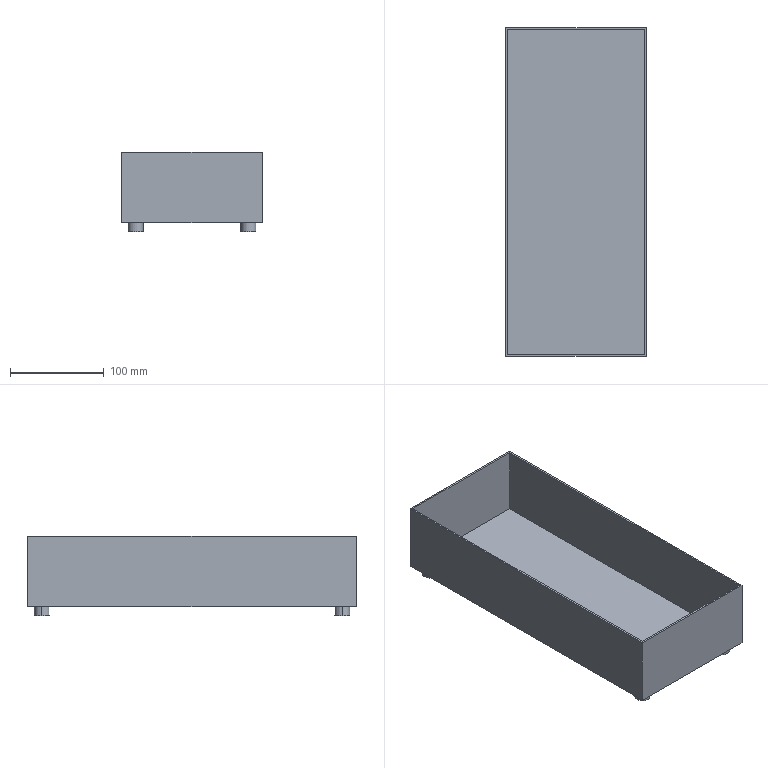Part | SolidWorks | features Extrusion 1, ICE 1, Shell 1 | 1 solid | 51 faces | box 150 x 350 x 85 mm | volume 254199 mm3 | plane 43 | cylinder 8 | commonest cylinder face diameters 16 x8
STEP:
#1=CARTESIAN_POINT('',(-68.,160.,-10.));
#2=VERTEX_POINT('',#1);
#3=CARTESIAN_POINT('',(-52.,160.,-10.));
#4=VERTEX_POINT('',#3);
#5=CARTESIAN_POINT('',(-60.,160.,-10.));
#6=DIRECTION('',(0.,0.,-1.));
#7=DIRECTION('',(1.,0.,0.));
#8=AXIS2_PLACEMENT_3D('',#5,#6,#7);
#9=CIRCLE('',#8,8.);
#10=EDGE_CURVE('',#2,#4,#9,.T.);
#11=ORIENTED_EDGE('',*,*,#10,.F.);
#12=CARTESIAN_POINT('',(-68.,160.,0.));
#13=VERTEX_POINT('',#12);
#14=CARTESIAN_POINT('',(-68.,160.,-10.));
#15=DIRECTION('',(0.,0.,1.));
#16=VECTOR('',#15,1000.);
#17=LINE('',#14,#16);
#18=EDGE_CURVE('',#2,#13,#17,.T.);
#19=ORIENTED_EDGE('',*,*,#18,.T.);
#20=CARTESIAN_POINT('',(-52.,160.,0.));
#21=VERTEX_POINT('',#20);
#22=CARTESIAN_POINT('',(-60.,160.,0.));
#23=DIRECTION('',(0.,0.,-1.));
#24=DIRECTION('',(1.,0.,0.));
#25=AXIS2_PLACEMENT_3D('',#22,#23,#24);
#26=CIRCLE('',#25,8.);
#27=EDGE_CURVE('',#13,#21,#26,.T.);
#28=ORIENTED_EDGE('',*,*,#27,.T.);
#29=CARTESIAN_POINT('',(-52.,160.,-10.));
#30=DIRECTION('',(0.,0.,1.));
#31=VECTOR('',#30,1000.);
#32=LINE('',#29,#31);
#33=EDGE_CURVE('',#4,#21,#32,.T.);
#34=ORIENTED_EDGE('',*,*,#33,.F.);
#35=EDGE_LOOP('',(#11,#19,#28,#34));
#36=FACE_OUTER_BOUND('',#35,.T.);
#37=CARTESIAN_POINT('',(-60.,160.,-10.));
#38=DIRECTION('',(0.,0.,1.));
#39=DIRECTION('',(1.,0.,0.));
#40=AXIS2_PLACEMENT_3D('',#37,#38,#39);
#41=CYLINDRICAL_SURFACE('',#40,8.);
#42=ADVANCED_FACE('',(#36),#41,.T.);
#43=CARTESIAN_POINT('',(-68.,-160.,-10.));
#44=VERTEX_POINT('',#43);
#45=CARTESIAN_POINT('',(-52.,-160.,-10.));
#46=VERTEX_POINT('',#45);
#47=CARTESIAN_POINT('',(-60.,-160.,-10.));
#48=DIRECTION('',(0.,0.,-1.));
#49=DIRECTION('',(-1.,0.,0.));
#50=AXIS2_PLACEMENT_3D('',#47,#48,#49);
#51=CIRCLE('',#50,8.);
#52=EDGE_CURVE('',#44,#46,#51,.T.);
#53=ORIENTED_EDGE('',*,*,#52,.F.);
#54=CARTESIAN_POINT('',(-68.,-160.,0.));
#55=VERTEX_POINT('',#54);
#56=CARTESIAN_POINT('',(-68.,-160.,-10.));
#57=DIRECTION('',(0.,0.,1.));
#58=VECTOR('',#57,1000.);
#59=LINE('',#56,#58);
#60=EDGE_CURVE('',#44,#55,#59,.T.);
#61=ORIENTED_EDGE('',*,*,#60,.T.);
#62=CARTESIAN_POINT('',(-52.,-160.,0.));
#63=VERTEX_POINT('',#62);
#64=CARTESIAN_POINT('',(-60.,-160.,0.));
#65=DIRECTION('',(0.,0.,-1.));
#66=DIRECTION('',(-1.,0.,0.));
#67=AXIS2_PLACEMENT_3D('',#64,#65,#66);
#68=CIRCLE('',#67,8.);
#69=EDGE_CURVE('',#55,#63,#68,.T.);
#70=ORIENTED_EDGE('',*,*,#69,.T.);
#71=CARTESIAN_POINT('',(-52.,-160.,-10.));
#72=DIRECTION('',(0.,0.,1.));
#73=VECTOR('',#72,1000.);
#74=LINE('',#71,#73);
#75=EDGE_CURVE('',#46,#63,#74,.T.);
#76=ORIENTED_EDGE('',*,*,#75,.F.);
#77=EDGE_LOOP('',(#53,#61,#70,#76));
#78=FACE_OUTER_BOUND('',#77,.T.);
#79=CARTESIAN_POINT('',(-60.,-160.,-10.));
#80=DIRECTION('',(0.,0.,1.));
#81=DIRECTION('',(1.,0.,0.));
#82=AXIS2_PLACEMENT_3D('',#79,#80,#81);
#83=CYLINDRICAL_SURFACE('',#82,8.);
#84=ADVANCED_FACE('',(#78),#83,.T.);
#85=CARTESIAN_POINT('',(52.,-160.,-10.));
#86=VERTEX_POINT('',#85);
#87=CARTESIAN_POINT('',(68.,-160.,-10.));
#88=VERTEX_POINT('',#87);
#89=CARTESIAN_POINT('',(60.,-160.,-10.));
#90=DIRECTION('',(0.,0.,-1.));
#91=DIRECTION('',(1.,0.,0.));
#92=AXIS2_PLACEMENT_3D('',#89,#90,#91);
#93=CIRCLE('',#92,8.);
#94=EDGE_CURVE('',#86,#88,#93,.T.);
#95=ORIENTED_EDGE('',*,*,#94,.F.);
#96=CARTESIAN_POINT('',(52.,-160.,0.));
#97=VERTEX_POINT('',#96);
#98=CARTESIAN_POINT('',(52.,-160.,-10.));
#99=DIRECTION('',(0.,0.,1.));
#100=VECTOR('',#99,1000.);
#101=LINE('',#98,#100);
#102=EDGE_CURVE('',#86,#97,#101,.T.);
#103=ORIENTED_EDGE('',*,*,#102,.T.);
#104=CARTESIAN_POINT('',(68.,-160.,0.));
#105=VERTEX_POINT('',#104);
#106=CARTESIAN_POINT('',(60.,-160.,0.));
#107=DIRECTION('',(0.,0.,-1.));
#108=DIRECTION('',(1.,0.,0.));
#109=AXIS2_PLACEMENT_3D('',#106,#107,#108);
#110=CIRCLE('',#109,8.);
#111=EDGE_CURVE('',#97,#105,#110,.T.);
#112=ORIENTED_EDGE('',*,*,#111,.T.);
#113=CARTESIAN_POINT('',(68.,-160.,-10.));
#114=DIRECTION('',(0.,0.,1.));
#115=VECTOR('',#114,1000.);
#116=LINE('',#113,#115);
#117=EDGE_CURVE('',#88,#105,#116,.T.);
#118=ORIENTED_EDGE('',*,*,#117,.F.);
#119=EDGE_LOOP('',(#95,#103,#112,#118));
#120=FACE_OUTER_BOUND('',#119,.T.);
#121=CARTESIAN_POINT('',(60.,-160.,-10.));
#122=DIRECTION('',(0.,0.,1.));
#123=DIRECTION('',(1.,0.,0.));
#124=AXIS2_PLACEMENT_3D('',#121,#122,#123);
#125=CYLINDRICAL_SURFACE('',#124,8.);
#126=ADVANCED_FACE('',(#120),#125,.T.);
#127=CARTESIAN_POINT('',(52.,160.,-10.));
#128=VERTEX_POINT('',#127);
#129=CARTESIAN_POINT('',(68.,160.,-10.));
#130=VERTEX_POINT('',#129);
#131=CARTESIAN_POINT('',(60.,160.,-10.));
#132=DIRECTION('',(0.,0.,-1.));
#133=DIRECTION('',(-1.,0.,0.));
#134=AXIS2_PLACEMENT_3D('',#131,#132,#133);
#135=CIRCLE('',#134,8.);
#136=EDGE_CURVE('',#128,#130,#135,.T.);
#137=ORIENTED_EDGE('',*,*,#136,.F.);
#138=CARTESIAN_POINT('',(52.,160.,0.));
#139=VERTEX_POINT('',#138);
#140=CARTESIAN_POINT('',(52.,160.,-10.));
#141=DIRECTION('',(0.,0.,1.));
#142=VECTOR('',#141,1000.);
#143=LINE('',#140,#142);
#144=EDGE_CURVE('',#128,#139,#143,.T.);
#145=ORIENTED_EDGE('',*,*,#144,.T.);
#146=CARTESIAN_POINT('',(68.,160.,0.));
#147=VERTEX_POINT('',#146);
#148=CARTESIAN_POINT('',(60.,160.,0.));
#149=DIRECTION('',(0.,0.,-1.));
#150=DIRECTION('',(-1.,0.,0.));
#151=AXIS2_PLACEMENT_3D('',#148,#149,#150);
#152=CIRCLE('',#151,8.);
#153=EDGE_CURVE('',#139,#147,#152,.T.);
#154=ORIENTED_EDGE('',*,*,#153,.T.);
#155=CARTESIAN_POINT('',(68.,160.,-10.));
#156=DIRECTION('',(0.,0.,1.));
#157=VECTOR('',#156,1000.);
#158=LINE('',#155,#157);
#159=EDGE_CURVE('',#130,#147,#158,.T.);
#160=ORIENTED_EDGE('',*,*,#159,.F.);
#161=EDGE_LOOP('',(#137,#145,#154,#160));
#162=FACE_OUTER_BOUND('',#161,.T.);
#163=CARTESIAN_POINT('',(60.,160.,-10.));
#164=DIRECTION('',(0.,0.,1.));
#165=DIRECTION('',(1.,0.,0.));
#166=AXIS2_PLACEMENT_3D('',#163,#164,#165);
#167=CYLINDRICAL_SURFACE('',#166,8.);
#168=ADVANCED_FACE('',(#162),#167,.T.);
#169=CARTESIAN_POINT('',(-60.,-160.,0.));
#170=DIRECTION('',(0.,0.,-1.));
#171=DIRECTION('',(-1.,0.,0.));
#172=AXIS2_PLACEMENT_3D('',#169,#170,#171);
#173=CIRCLE('',#172,8.);
#174=EDGE_CURVE('',#63,#55,#173,.T.);
#175=ORIENTED_EDGE('',*,*,#174,.F.);
#176=ORIENTED_EDGE('',*,*,#69,.F.);
#177=EDGE_LOOP('',(#175,#176));
#178=FACE_BOUND('',#177,.T.);
#179=CARTESIAN_POINT('',(60.,160.,0.));
#180=DIRECTION('',(0.,0.,-1.));
#181=DIRECTION('',(-1.,0.,0.));
#182=AXIS2_PLACEMENT_3D('',#179,#180,#181);
#183=CIRCLE('',#182,8.);
#184=EDGE_CURVE('',#147,#139,#183,.T.);
#185=ORIENTED_EDGE('',*,*,#184,.F.);
#186=ORIENTED_EDGE('',*,*,#153,.F.);
#187=EDGE_LOOP('',(#185,#186));
#188=FACE_BOUND('',#187,.T.);
#189=CARTESIAN_POINT('',(-75.,175.,0.));
#190=VERTEX_POINT('',#189);
#191=CARTESIAN_POINT('',(-75.,-175.,0.));
#192=VERTEX_POINT('',#191);
#193=CARTESIAN_POINT('',(-75.,175.,0.));
#194=DIRECTION('',(0.,-1.,0.));
#195=VECTOR('',#194,1000.);
#196=LINE('',#193,#195);
#197=EDGE_CURVE('',#190,#192,#196,.T.);
#198=ORIENTED_EDGE('',*,*,#197,.F.);
#199=CARTESIAN_POINT('',(75.,175.,0.));
#200=VERTEX_POINT('',#199);
#201=CARTESIAN_POINT('',(75.,175.,0.));
#202=DIRECTION('',(-1.,0.,0.));
#203=VECTOR('',#202,1000.);
#204=LINE('',#201,#203);
#205=EDGE_CURVE('',#200,#190,#204,.T.);
#206=ORIENTED_EDGE('',*,*,#205,.F.);
#207=CARTESIAN_POINT('',(75.,-175.,0.));
#208=VERTEX_POINT('',#207);
#209=CARTESIAN_POINT('',(75.,175.,0.));
#210=DIRECTION('',(0.,1.,0.));
#211=VECTOR('',#210,1000.);
#212=LINE('',#209,#211);
#213=EDGE_CURVE('',#208,#200,#212,.T.);
#214=ORIENTED_EDGE('',*,*,#213,.F.);
#215=CARTESIAN_POINT('',(75.,-175.,0.));
#216=DIRECTION('',(1.,0.,0.));
#217=VECTOR('',#216,1000.);
#218=LINE('',#215,#217);
#219=EDGE_CURVE('',#192,#208,#218,.T.);
#220=ORIENTED_EDGE('',*,*,#219,.F.);
#221=EDGE_LOOP('',(#198,#206,#214,#220));
#222=FACE_OUTER_BOUND('',#221,.T.);
#223=CARTESIAN_POINT('',(60.,-160.,0.));
#224=DIRECTION('',(0.,0.,-1.));
#225=DIRECTION('',(1.,0.,0.));
#226=AXIS2_PLACEMENT_3D('',#223,#224,#225);
#227=CIRCLE('',#226,8.);
#228=EDGE_CURVE('',#105,#97,#227,.T.);
#229=ORIENTED_EDGE('',*,*,#228,.F.);
#230=ORIENTED_EDGE('',*,*,#111,.F.);
#231=EDGE_LOOP('',(#229,#230));
#232=FACE_BOUND('',#231,.T.);
#233=CARTESIAN_POINT('',(-60.,160.,0.));
#234=DIRECTION('',(0.,0.,-1.));
#235=DIRECTION('',(1.,0.,0.));
#236=AXIS2_PLACEMENT_3D('',#233,#234,#235);
#237=CIRCLE('',#236,8.);
#238=EDGE_CURVE('',#21,#13,#237,.T.);
#239=ORIENTED_EDGE('',*,*,#238,.F.);
#240=ORIENTED_EDGE('',*,*,#27,.F.);
#241=EDGE_LOOP('',(#239,#240));
#242=FACE_BOUND('',#241,.T.);
#243=CARTESIAN_POINT('',(0.,0.,0.));
#244=DIRECTION('',(0.,0.,-1.));
#245=DIRECTION('',(-1.,0.,0.));
#246=AXIS2_PLACEMENT_3D('',#243,#244,#245);
#247=PLANE('',#246);
#248=ADVANCED_FACE('',(#178,#188,#222,#232,#242),#247,.T.);
#249=CARTESIAN_POINT('',(-75.,175.,75.));
#250=VERTEX_POINT('',#249);
#251=CARTESIAN_POINT('',(-75.,-175.,75.));
#252=VERTEX_POINT('',#251);
#253=CARTESIAN_POINT('',(-75.,175.,75.));
#254=DIRECTION('',(0.,-1.,0.));
#255=VECTOR('',#254,1000.);
#256=LINE('',#253,#255);
#257=EDGE_CURVE('',#250,#252,#256,.T.);
#258=ORIENTED_EDGE('',*,*,#257,.T.);
#259=CARTESIAN_POINT('',(75.,-175.,75.));
#260=VERTEX_POINT('',#259);
#261=CARTESIAN_POINT('',(75.,-175.,75.));
#262=DIRECTION('',(1.,0.,0.));
#263=VECTOR('',#262,1000.);
#264=LINE('',#261,#263);
#265=EDGE_CURVE('',#252,#260,#264,.T.);
#266=ORIENTED_EDGE('',*,*,#265,.T.);
#267=CARTESIAN_POINT('',(75.,175.,75.));
#268=VERTEX_POINT('',#267);
#269=CARTESIAN_POINT('',(75.,175.,75.));
#270=DIRECTION('',(0.,1.,0.));
#271=VECTOR('',#270,1000.);
#272=LINE('',#269,#271);
#273=EDGE_CURVE('',#260,#268,#272,.T.);
#274=ORIENTED_EDGE('',*,*,#273,.T.);
#275=CARTESIAN_POINT('',(75.,175.,75.));
#276=DIRECTION('',(-1.,0.,0.));
#277=VECTOR('',#276,1000.);
#278=LINE('',#275,#277);
#279=EDGE_CURVE('',#268,#250,#278,.T.);
#280=ORIENTED_EDGE('',*,*,#279,.T.);
#281=EDGE_LOOP('',(#258,#266,#274,#280));
#282=FACE_OUTER_BOUND('',#281,.T.);
#283=CARTESIAN_POINT('',(-73.,173.,75.));
#284=VERTEX_POINT('',#283);
#285=CARTESIAN_POINT('',(-73.,-173.,75.));
#286=VERTEX_POINT('',#285);
#287=CARTESIAN_POINT('',(-73.,0.,75.));
#288=DIRECTION('',(0.,-1.,0.));
#289=VECTOR('',#288,1000.);
#290=LINE('',#287,#289);
#291=EDGE_CURVE('',#284,#286,#290,.T.);
#292=ORIENTED_EDGE('',*,*,#291,.F.);
#293=CARTESIAN_POINT('',(73.,173.,75.));
#294=VERTEX_POINT('',#293);
#295=CARTESIAN_POINT('',(0.,173.,75.));
#296=DIRECTION('',(-1.,0.,0.));
#297=VECTOR('',#296,1000.);
#298=LINE('',#295,#297);
#299=EDGE_CURVE('',#294,#284,#298,.T.);
#300=ORIENTED_EDGE('',*,*,#299,.F.);
#301=CARTESIAN_POINT('',(73.,-173.,75.));
#302=VERTEX_POINT('',#301);
#303=CARTESIAN_POINT('',(73.,0.,75.));
#304=DIRECTION('',(0.,1.,0.));
#305=VECTOR('',#304,1000.);
#306=LINE('',#303,#305);
#307=EDGE_CURVE('',#302,#294,#306,.T.);
#308=ORIENTED_EDGE('',*,*,#307,.F.);
#309=CARTESIAN_POINT('',(0.,-173.,75.));
#310=DIRECTION('',(1.,0.,0.));
#311=VECTOR('',#310,1000.);
#312=LINE('',#309,#311);
#313=EDGE_CURVE('',#286,#302,#312,.T.);
#314=ORIENTED_EDGE('',*,*,#313,.F.);
#315=EDGE_LOOP('',(#292,#300,#308,#314));
#316=FACE_BOUND('',#315,.T.);
#317=CARTESIAN_POINT('',(0.,0.,75.));
#318=DIRECTION('',(0.,0.,-1.));
#319=DIRECTION('',(-1.,0.,0.));
#320=AXIS2_PLACEMENT_3D('',#317,#318,#319);
#321=PLANE('',#320);
#322=ADVANCED_FACE('',(#282,#316),#321,.F.);
#323=ORIENTED_EDGE('',*,*,#197,.T.);
#324=CARTESIAN_POINT('',(-75.,-175.,75.));
#325=DIRECTION('',(0.,0.,-1.));
#326=VECTOR('',#325,1000.);
#327=LINE('',#324,#326);
#328=EDGE_CURVE('',#252,#192,#327,.T.);
#329=ORIENTED_EDGE('',*,*,#328,.F.);
#330=ORIENTED_EDGE('',*,*,#257,.F.);
#331=CARTESIAN_POINT('',(-75.,175.,75.));
#332=DIRECTION('',(0.,0.,-1.));
#333=VECTOR('',#332,1000.);
#334=LINE('',#331,#333);
#335=EDGE_CURVE('',#250,#190,#334,.T.);
#336=ORIENTED_EDGE('',*,*,#335,.T.);
#337=EDGE_LOOP('',(#323,#329,#330,#336));
#338=FACE_OUTER_BOUND('',#337,.T.);
#339=CARTESIAN_POINT('',(-75.,175.,75.));
#340=DIRECTION('',(1.,0.,0.));
#341=DIRECTION('',(0.,1.,0.));
#342=AXIS2_PLACEMENT_3D('',#339,#340,#341);
#343=PLANE('',#342);
#344=ADVANCED_FACE('',(#338),#343,.F.);
#345=ORIENTED_EDGE('',*,*,#219,.T.);
#346=CARTESIAN_POINT('',(75.,-175.,75.));
#347=DIRECTION('',(0.,0.,-1.));
#348=VECTOR('',#347,1000.);
#349=LINE('',#346,#348);
#350=EDGE_CURVE('',#260,#208,#349,.T.);
#351=ORIENTED_EDGE('',*,*,#350,.F.);
#352=ORIENTED_EDGE('',*,*,#265,.F.);
#353=ORIENTED_EDGE('',*,*,#328,.T.);
#354=EDGE_LOOP('',(#345,#351,#352,#353));
#355=FACE_OUTER_BOUND('',#354,.T.);
#356=CARTESIAN_POINT('',(75.,-175.,75.));
#357=DIRECTION('',(0.,1.,0.));
#358=DIRECTION('',(0.,0.,1.));
#359=AXIS2_PLACEMENT_3D('',#356,#357,#358);
#360=PLANE('',#359);
#361=ADVANCED_FACE('',(#355),#360,.F.);
#362=ORIENTED_EDGE('',*,*,#213,.T.);
#363=CARTESIAN_POINT('',(75.,175.,75.));
#364=DIRECTION('',(0.,0.,-1.));
#365=VECTOR('',#364,1000.);
#366=LINE('',#363,#365);
#367=EDGE_CURVE('',#268,#200,#366,.T.);
#368=ORIENTED_EDGE('',*,*,#367,.F.);
#369=ORIENTED_EDGE('',*,*,#273,.F.);
#370=ORIENTED_EDGE('',*,*,#350,.T.);
#371=EDGE_LOOP('',(#362,#368,#369,#370));
#372=FACE_OUTER_BOUND('',#371,.T.);
#373=CARTESIAN_POINT('',(75.,175.,75.));
#374=DIRECTION('',(-1.,0.,0.));
#375=DIRECTION('',(0.,-1.,0.));
#376=AXIS2_PLACEMENT_3D('',#373,#374,#375);
#377=PLANE('',#376);
#378=ADVANCED_FACE('',(#372),#377,.F.);
#379=ORIENTED_EDGE('',*,*,#205,.T.);
#380=ORIENTED_EDGE('',*,*,#335,.F.);
#381=ORIENTED_EDGE('',*,*,#279,.F.);
#382=ORIENTED_EDGE('',*,*,#367,.T.);
#383=EDGE_LOOP('',(#379,#380,#381,#382));
#384=FACE_OUTER_BOUND('',#383,.T.);
#385=CARTESIAN_POINT('',(75.,175.,75.));
#386=DIRECTION('',(0.,-1.,0.));
#387=DIRECTION('',(0.,0.,-1.));
#388=AXIS2_PLACEMENT_3D('',#385,#386,#387);
#389=PLANE('',#388);
#390=ADVANCED_FACE('',(#384),#389,.F.);
#391=CARTESIAN_POINT('',(-73.,173.,2.));
#392=VERTEX_POINT('',#391);
#393=CARTESIAN_POINT('',(-73.,-173.,2.));
#394=VERTEX_POINT('',#393);
#395=CARTESIAN_POINT('',(-73.,0.,2.));
#396=DIRECTION('',(0.,-1.,0.));
#397=VECTOR('',#396,1000.);
#398=LINE('',#395,#397);
#399=EDGE_CURVE('',#392,#394,#398,.T.);
#400=ORIENTED_EDGE('',*,*,#399,.F.);
#401=CARTESIAN_POINT('',(-73.,173.,75.));
#402=DIRECTION('',(0.,0.,-1.));
#403=VECTOR('',#402,1000.);
#404=LINE('',#401,#403);
#405=EDGE_CURVE('',#284,#392,#404,.T.);
#406=ORIENTED_EDGE('',*,*,#405,.F.);
#407=ORIENTED_EDGE('',*,*,#291,.T.);
#408=CARTESIAN_POINT('',(-73.,-173.,75.));
#409=DIRECTION('',(0.,0.,-1.));
#410=VECTOR('',#409,1000.);
#411=LINE('',#408,#410);
#412=EDGE_CURVE('',#286,#394,#411,.T.);
#413=ORIENTED_EDGE('',*,*,#412,.T.);
#414=EDGE_LOOP('',(#400,#406,#407,#413));
#415=FACE_OUTER_BOUND('',#414,.T.);
#416=CARTESIAN_POINT('',(-73.,175.,75.));
#417=DIRECTION('',(1.,0.,0.));
#418=DIRECTION('',(0.,1.,0.));
#419=AXIS2_PLACEMENT_3D('',#416,#417,#418);
#420=PLANE('',#419);
#421=ADVANCED_FACE('',(#415),#420,.T.);
#422=CARTESIAN_POINT('',(73.,-173.,2.));
#423=VERTEX_POINT('',#422);
#424=CARTESIAN_POINT('',(0.,-173.,2.));
#425=DIRECTION('',(1.,0.,0.));
#426=VECTOR('',#425,1000.);
#427=LINE('',#424,#426);
#428=EDGE_CURVE('',#394,#423,#427,.T.);
#429=ORIENTED_EDGE('',*,*,#428,.F.);
#430=ORIENTED_EDGE('',*,*,#412,.F.);
#431=ORIENTED_EDGE('',*,*,#313,.T.);
#432=CARTESIAN_POINT('',(73.,-173.,75.));
#433=DIRECTION('',(0.,0.,-1.));
#434=VECTOR('',#433,1000.);
#435=LINE('',#432,#434);
#436=EDGE_CURVE('',#302,#423,#435,.T.);
#437=ORIENTED_EDGE('',*,*,#436,.T.);
#438=EDGE_LOOP('',(#429,#430,#431,#437));
#439=FACE_OUTER_BOUND('',#438,.T.);
#440=CARTESIAN_POINT('',(75.,-173.,75.));
#441=DIRECTION('',(0.,1.,0.));
#442=DIRECTION('',(0.,0.,1.));
#443=AXIS2_PLACEMENT_3D('',#440,#441,#442);
#444=PLANE('',#443);
#445=ADVANCED_FACE('',(#439),#444,.T.);
#446=CARTESIAN_POINT('',(73.,173.,2.));
#447=VERTEX_POINT('',#446);
#448=CARTESIAN_POINT('',(73.,0.,2.));
#449=DIRECTION('',(0.,1.,0.));
#450=VECTOR('',#449,1000.);
#451=LINE('',#448,#450);
#452=EDGE_CURVE('',#423,#447,#451,.T.);
#453=ORIENTED_EDGE('',*,*,#452,.F.);
#454=ORIENTED_EDGE('',*,*,#436,.F.);
#455=ORIENTED_EDGE('',*,*,#307,.T.);
#456=CARTESIAN_POINT('',(73.,173.,75.));
#457=DIRECTION('',(0.,0.,-1.));
#458=VECTOR('',#457,1000.);
#459=LINE('',#456,#458);
#460=EDGE_CURVE('',#294,#447,#459,.T.);
#461=ORIENTED_EDGE('',*,*,#460,.T.);
#462=EDGE_LOOP('',(#453,#454,#455,#461));
#463=FACE_OUTER_BOUND('',#462,.T.);
#464=CARTESIAN_POINT('',(73.,175.,75.));
#465=DIRECTION('',(-1.,0.,0.));
#466=DIRECTION('',(0.,-1.,0.));
#467=AXIS2_PLACEMENT_3D('',#464,#465,#466);
#468=PLANE('',#467);
#469=ADVANCED_FACE('',(#463),#468,.T.);
#470=CARTESIAN_POINT('',(0.,173.,2.));
#471=DIRECTION('',(-1.,0.,0.));
#472=VECTOR('',#471,1000.);
#473=LINE('',#470,#472);
#474=EDGE_CURVE('',#447,#392,#473,.T.);
#475=ORIENTED_EDGE('',*,*,#474,.F.);
#476=ORIENTED_EDGE('',*,*,#460,.F.);
#477=ORIENTED_EDGE('',*,*,#299,.T.);
#478=ORIENTED_EDGE('',*,*,#405,.T.);
#479=EDGE_LOOP('',(#475,#476,#477,#478));
#480=FACE_OUTER_BOUND('',#479,.T.);
#481=CARTESIAN_POINT('',(75.,173.,75.));
#482=DIRECTION('',(0.,-1.,0.));
#483=DIRECTION('',(0.,0.,-1.));
#484=AXIS2_PLACEMENT_3D('',#481,#482,#483);
#485=PLANE('',#484);
#486=ADVANCED_FACE('',(#480),#485,.T.);
#487=ORIENTED_EDGE('',*,*,#399,.T.);
#488=ORIENTED_EDGE('',*,*,#428,.T.);
#489=ORIENTED_EDGE('',*,*,#452,.T.);
#490=ORIENTED_EDGE('',*,*,#474,.T.);
#491=EDGE_LOOP('',(#487,#488,#489,#490));
#492=FACE_OUTER_BOUND('',#491,.T.);
#493=CARTESIAN_POINT('',(0.,0.,2.));
#494=DIRECTION('',(0.,0.,-1.));
#495=DIRECTION('',(-1.,0.,0.));
#496=AXIS2_PLACEMENT_3D('',#493,#494,#495);
#497=PLANE('',#496);
#498=ADVANCED_FACE('',(#492),#497,.F.);
#499=CARTESIAN_POINT('',(60.,160.,-10.));
#500=DIRECTION('',(0.,0.,-1.));
#501=DIRECTION('',(-1.,0.,0.));
#502=AXIS2_PLACEMENT_3D('',#499,#500,#501);
#503=CIRCLE('',#502,8.);
#504=EDGE_CURVE('',#130,#128,#503,.T.);
#505=ORIENTED_EDGE('',*,*,#504,.T.);
#506=ORIENTED_EDGE('',*,*,#136,.T.);
#507=EDGE_LOOP('',(#505,#506));
#508=FACE_OUTER_BOUND('',#507,.T.);
#509=CARTESIAN_POINT('',(62.973,154.85,-10.));
#510=VERTEX_POINT('',#509);
#511=CARTESIAN_POINT('',(57.027,154.85,-10.));
#512=VERTEX_POINT('',#511);
#513=CARTESIAN_POINT('',(62.973,154.85,-10.));
#514=DIRECTION('',(-1.,0.,0.));
#515=VECTOR('',#514,1000.);
#516=LINE('',#513,#515);
#517=EDGE_CURVE('',#510,#512,#516,.T.);
#518=ORIENTED_EDGE('',*,*,#517,.F.);
#519=CARTESIAN_POINT('',(65.947,160.,-10.));
#520=VERTEX_POINT('',#519);
#521=CARTESIAN_POINT('',(65.947,160.,-10.));
#522=DIRECTION('',(-0.5,-0.866,0.));
#523=VECTOR('',#522,1000.);
#524=LINE('',#521,#523);
#525=EDGE_CURVE('',#520,#510,#524,.T.);
#526=ORIENTED_EDGE('',*,*,#525,.F.);
#527=CARTESIAN_POINT('',(62.973,165.15,-10.));
#528=VERTEX_POINT('',#527);
#529=CARTESIAN_POINT('',(62.973,165.15,-10.));
#530=DIRECTION('',(0.5,-0.866,0.));
#531=VECTOR('',#530,1000.);
#532=LINE('',#529,#531);
#533=EDGE_CURVE('',#528,#520,#532,.T.);
#534=ORIENTED_EDGE('',*,*,#533,.F.);
#535=CARTESIAN_POINT('',(57.027,165.15,-10.));
#536=VERTEX_POINT('',#535);
#537=CARTESIAN_POINT('',(57.027,165.15,-10.));
#538=DIRECTION('',(1.,0.,0.));
#539=VECTOR('',#538,1000.);
#540=LINE('',#537,#539);
#541=EDGE_CURVE('',#536,#528,#540,.T.);
#542=ORIENTED_EDGE('',*,*,#541,.F.);
#543=CARTESIAN_POINT('',(54.053,160.,-10.));
#544=VERTEX_POINT('',#543);
#545=CARTESIAN_POINT('',(54.053,160.,-10.));
#546=DIRECTION('',(0.5,0.866,0.));
#547=VECTOR('',#546,1000.);
#548=LINE('',#545,#547);
#549=EDGE_CURVE('',#544,#536,#548,.T.);
#550=ORIENTED_EDGE('',*,*,#549,.F.);
#551=CARTESIAN_POINT('',(57.027,154.85,-10.));
#552=DIRECTION('',(-0.5,0.866,0.));
#553=VECTOR('',#552,1000.);
#554=LINE('',#551,#553);
#555=EDGE_CURVE('',#512,#544,#554,.T.);
#556=ORIENTED_EDGE('',*,*,#555,.F.);
#557=EDGE_LOOP('',(#518,#526,#534,#542,#550,#556));
#558=FACE_BOUND('',#557,.T.);
#559=CARTESIAN_POINT('',(60.,160.,-10.));
#560=DIRECTION('',(0.,0.,-1.));
#561=DIRECTION('',(-1.,0.,0.));
#562=AXIS2_PLACEMENT_3D('',#559,#560,#561);
#563=PLANE('',#562);
#564=ADVANCED_FACE('',(#508,#558),#563,.T.);
#565=ORIENTED_EDGE('',*,*,#144,.F.);
#566=ORIENTED_EDGE('',*,*,#504,.F.);
#567=ORIENTED_EDGE('',*,*,#159,.T.);
#568=ORIENTED_EDGE('',*,*,#184,.T.);
#569=EDGE_LOOP('',(#565,#566,#567,#568));
#570=FACE_OUTER_BOUND('',#569,.T.);
#571=CARTESIAN_POINT('',(60.,160.,-10.));
#572=DIRECTION('',(0.,0.,1.));
#573=DIRECTION('',(1.,0.,0.));
#574=AXIS2_PLACEMENT_3D('',#571,#572,#573);
#575=CYLINDRICAL_SURFACE('',#574,8.);
#576=ADVANCED_FACE('',(#570),#575,.T.);
#577=CARTESIAN_POINT('',(65.947,160.,0.));
#578=VERTEX_POINT('',#577);
#579=CARTESIAN_POINT('',(62.973,154.85,0.));
#580=VERTEX_POINT('',#579);
#581=CARTESIAN_POINT('',(65.947,160.,0.));
#582=DIRECTION('',(-0.5,-0.866,0.));
#583=VECTOR('',#582,1000.);
#584=LINE('',#581,#583);
#585=EDGE_CURVE('',#578,#580,#584,.T.);
#586=ORIENTED_EDGE('',*,*,#585,.F.);
#587=CARTESIAN_POINT('',(65.947,160.,-10.));
#588=DIRECTION('',(0.,0.,1.));
#589=VECTOR('',#588,1000.);
#590=LINE('',#587,#589);
#591=EDGE_CURVE('',#520,#578,#590,.T.);
#592=ORIENTED_EDGE('',*,*,#591,.F.);
#593=ORIENTED_EDGE('',*,*,#525,.T.);
#594=CARTESIAN_POINT('',(62.973,154.85,-10.));
#595=DIRECTION('',(0.,0.,1.));
#596=VECTOR('',#595,1000.);
#597=LINE('',#594,#596);
#598=EDGE_CURVE('',#510,#580,#597,.T.);
#599=ORIENTED_EDGE('',*,*,#598,.T.);
#600=EDGE_LOOP('',(#586,#592,#593,#599));
#601=FACE_OUTER_BOUND('',#600,.T.);
#602=CARTESIAN_POINT('',(65.947,160.,-10.));
#603=DIRECTION('',(-0.866,0.5,0.));
#604=DIRECTION('',(-0.5,-0.866,0.));
#605=AXIS2_PLACEMENT_3D('',#602,#603,#604);
#606=PLANE('',#605);
#607=ADVANCED_FACE('',(#601),#606,.T.);
#608=CARTESIAN_POINT('',(57.027,154.85,0.));
#609=VERTEX_POINT('',#608);
#610=CARTESIAN_POINT('',(62.973,154.85,0.));
#611=DIRECTION('',(-1.,0.,0.));
#612=VECTOR('',#611,1000.);
#613=LINE('',#610,#612);
#614=EDGE_CURVE('',#580,#609,#613,.T.);
#615=ORIENTED_EDGE('',*,*,#614,.F.);
#616=ORIENTED_EDGE('',*,*,#598,.F.);
#617=ORIENTED_EDGE('',*,*,#517,.T.);
#618=CARTESIAN_POINT('',(57.027,154.85,-10.));
#619=DIRECTION('',(0.,0.,1.));
#620=VECTOR('',#619,1000.);
#621=LINE('',#618,#620);
#622=EDGE_CURVE('',#512,#609,#621,.T.);
#623=ORIENTED_EDGE('',*,*,#622,.T.);
#624=EDGE_LOOP('',(#615,#616,#617,#623));
#625=FACE_OUTER_BOUND('',#624,.T.);
#626=CARTESIAN_POINT('',(62.973,154.85,-10.));
#627=DIRECTION('',(0.,1.,0.));
#628=DIRECTION('',(-1.,0.,0.));
#629=AXIS2_PLACEMENT_3D('',#626,#627,#628);
#630=PLANE('',#629);
#631=ADVANCED_FACE('',(#625),#630,.T.);
#632=CARTESIAN_POINT('',(54.053,160.,0.));
#633=VERTEX_POINT('',#632);
#634=CARTESIAN_POINT('',(57.027,154.85,0.));
#635=DIRECTION('',(-0.5,0.866,0.));
#636=VECTOR('',#635,1000.);
#637=LINE('',#634,#636);
#638=EDGE_CURVE('',#609,#633,#637,.T.);
#639=ORIENTED_EDGE('',*,*,#638,.F.);
#640=ORIENTED_EDGE('',*,*,#622,.F.);
#641=ORIENTED_EDGE('',*,*,#555,.T.);
#642=CARTESIAN_POINT('',(54.053,160.,-10.));
#643=DIRECTION('',(0.,0.,1.));
#644=VECTOR('',#643,1000.);
#645=LINE('',#642,#644);
#646=EDGE_CURVE('',#544,#633,#645,.T.);
#647=ORIENTED_EDGE('',*,*,#646,.T.);
#648=EDGE_LOOP('',(#639,#640,#641,#647));
#649=FACE_OUTER_BOUND('',#648,.T.);
#650=CARTESIAN_POINT('',(57.027,154.85,-10.));
#651=DIRECTION('',(0.866,0.5,0.));
#652=DIRECTION('',(-0.5,0.866,0.));
#653=AXIS2_PLACEMENT_3D('',#650,#651,#652);
#654=PLANE('',#653);
#655=ADVANCED_FACE('',(#649),#654,.T.);
#656=CARTESIAN_POINT('',(57.027,165.15,0.));
#657=VERTEX_POINT('',#656);
#658=CARTESIAN_POINT('',(54.053,160.,0.));
#659=DIRECTION('',(0.5,0.866,0.));
#660=VECTOR('',#659,1000.);
#661=LINE('',#658,#660);
#662=EDGE_CURVE('',#633,#657,#661,.T.);
#663=ORIENTED_EDGE('',*,*,#662,.F.);
#664=ORIENTED_EDGE('',*,*,#646,.F.);
#665=ORIENTED_EDGE('',*,*,#549,.T.);
#666=CARTESIAN_POINT('',(57.027,165.15,-10.));
#667=DIRECTION('',(0.,0.,1.));
#668=VECTOR('',#667,1000.);
#669=LINE('',#666,#668);
#670=EDGE_CURVE('',#536,#657,#669,.T.);
#671=ORIENTED_EDGE('',*,*,#670,.T.);
#672=EDGE_LOOP('',(#663,#664,#665,#671));
#673=FACE_OUTER_BOUND('',#672,.T.);
#674=CARTESIAN_POINT('',(54.053,160.,-10.));
#675=DIRECTION('',(0.866,-0.5,0.));
#676=DIRECTION('',(0.5,0.866,0.));
#677=AXIS2_PLACEMENT_3D('',#674,#675,#676);
#678=PLANE('',#677);
#679=ADVANCED_FACE('',(#673),#678,.T.);
#680=CARTESIAN_POINT('',(62.973,165.15,0.));
#681=VERTEX_POINT('',#680);
#682=CARTESIAN_POINT('',(57.027,165.15,0.));
#683=DIRECTION('',(1.,0.,0.));
#684=VECTOR('',#683,1000.);
#685=LINE('',#682,#684);
#686=EDGE_CURVE('',#657,#681,#685,.T.);
#687=ORIENTED_EDGE('',*,*,#686,.F.);
#688=ORIENTED_EDGE('',*,*,#670,.F.);
#689=ORIENTED_EDGE('',*,*,#541,.T.);
#690=CARTESIAN_POINT('',(62.973,165.15,-10.));
#691=DIRECTION('',(0.,0.,1.));
#692=VECTOR('',#691,1000.);
#693=LINE('',#690,#692);
#694=EDGE_CURVE('',#528,#681,#693,.T.);
#695=ORIENTED_EDGE('',*,*,#694,.T.);
#696=EDGE_LOOP('',(#687,#688,#689,#695));
#697=FACE_OUTER_BOUND('',#696,.T.);
#698=CARTESIAN_POINT('',(57.027,165.15,-10.));
#699=DIRECTION('',(0.,-1.,0.));
#700=DIRECTION('',(0.,0.,-1.));
#701=AXIS2_PLACEMENT_3D('',#698,#699,#700);
#702=PLANE('',#701);
#703=ADVANCED_FACE('',(#697),#702,.T.);
#704=CARTESIAN_POINT('',(62.973,165.15,0.));
#705=DIRECTION('',(0.5,-0.866,0.));
#706=VECTOR('',#705,1000.);
#707=LINE('',#704,#706);
#708=EDGE_CURVE('',#681,#578,#707,.T.);
#709=ORIENTED_EDGE('',*,*,#708,.F.);
#710=ORIENTED_EDGE('',*,*,#694,.F.);
#711=ORIENTED_EDGE('',*,*,#533,.T.);
#712=ORIENTED_EDGE('',*,*,#591,.T.);
#713=EDGE_LOOP('',(#709,#710,#711,#712));
#714=FACE_OUTER_BOUND('',#713,.T.);
#715=CARTESIAN_POINT('',(62.973,165.15,-10.));
#716=DIRECTION('',(-0.866,-0.5,0.));
#717=DIRECTION('',(0.5,-0.866,0.));
#718=AXIS2_PLACEMENT_3D('',#715,#716,#717);
#719=PLANE('',#718);
#720=ADVANCED_FACE('',(#714),#719,.T.);
#721=ORIENTED_EDGE('',*,*,#585,.T.);
#722=ORIENTED_EDGE('',*,*,#614,.T.);
#723=ORIENTED_EDGE('',*,*,#638,.T.);
#724=ORIENTED_EDGE('',*,*,#662,.T.);
#725=ORIENTED_EDGE('',*,*,#686,.T.);
#726=ORIENTED_EDGE('',*,*,#708,.T.);
#727=EDGE_LOOP('',(#721,#722,#723,#724,#725,#726));
#728=FACE_OUTER_BOUND('',#727,.T.);
#729=CARTESIAN_POINT('',(0.,0.,0.));
#730=DIRECTION('',(0.,0.,-1.));
#731=DIRECTION('',(-1.,0.,0.));
#732=AXIS2_PLACEMENT_3D('',#729,#730,#731);
#733=PLANE('',#732);
#734=ADVANCED_FACE('',(#728),#733,.T.);
#735=CARTESIAN_POINT('',(60.,-160.,-10.));
#736=DIRECTION('',(0.,0.,-1.));
#737=DIRECTION('',(1.,0.,0.));
#738=AXIS2_PLACEMENT_3D('',#735,#736,#737);
#739=CIRCLE('',#738,8.);
#740=EDGE_CURVE('',#88,#86,#739,.T.);
#741=ORIENTED_EDGE('',*,*,#740,.T.);
#742=ORIENTED_EDGE('',*,*,#94,.T.);
#743=EDGE_LOOP('',(#741,#742));
#744=FACE_OUTER_BOUND('',#743,.T.);
#745=CARTESIAN_POINT('',(65.947,-160.,-10.));
#746=VERTEX_POINT('',#745);
#747=CARTESIAN_POINT('',(62.973,-165.15,-10.));
#748=VERTEX_POINT('',#747);
#749=CARTESIAN_POINT('',(62.973,-165.15,-10.));
#750=DIRECTION('',(-0.5,-0.866,0.));
#751=VECTOR('',#750,1000.);
#752=LINE('',#749,#751);
#753=EDGE_CURVE('',#746,#748,#752,.T.);
#754=ORIENTED_EDGE('',*,*,#753,.F.);
#755=CARTESIAN_POINT('',(62.973,-154.85,-10.));
#756=VERTEX_POINT('',#755);
#757=CARTESIAN_POINT('',(65.947,-160.,-10.));
#758=DIRECTION('',(0.5,-0.866,0.));
#759=VECTOR('',#758,1000.);
#760=LINE('',#757,#759);
#761=EDGE_CURVE('',#756,#746,#760,.T.);
#762=ORIENTED_EDGE('',*,*,#761,.F.);
#763=CARTESIAN_POINT('',(57.027,-154.85,-10.));
#764=VERTEX_POINT('',#763);
#765=CARTESIAN_POINT('',(62.973,-154.85,-10.));
#766=DIRECTION('',(1.,0.,0.));
#767=VECTOR('',#766,1000.);
#768=LINE('',#765,#767);
#769=EDGE_CURVE('',#764,#756,#768,.T.);
#770=ORIENTED_EDGE('',*,*,#769,.F.);
#771=CARTESIAN_POINT('',(54.053,-160.,-10.));
#772=VERTEX_POINT('',#771);
#773=CARTESIAN_POINT('',(57.027,-154.85,-10.));
#774=DIRECTION('',(0.5,0.866,0.));
#775=VECTOR('',#774,1000.);
#776=LINE('',#773,#775);
#777=EDGE_CURVE('',#772,#764,#776,.T.);
#778=ORIENTED_EDGE('',*,*,#777,.F.);
#779=CARTESIAN_POINT('',(57.027,-165.15,-10.));
#780=VERTEX_POINT('',#779);
#781=CARTESIAN_POINT('',(54.053,-160.,-10.));
#782=DIRECTION('',(-0.5,0.866,0.));
#783=VECTOR('',#782,1000.);
#784=LINE('',#781,#783);
#785=EDGE_CURVE('',#780,#772,#784,.T.);
#786=ORIENTED_EDGE('',*,*,#785,.F.);
#787=CARTESIAN_POINT('',(57.027,-165.15,-10.));
#788=DIRECTION('',(-1.,0.,0.));
#789=VECTOR('',#788,1000.);
#790=LINE('',#787,#789);
#791=EDGE_CURVE('',#748,#780,#790,.T.);
#792=ORIENTED_EDGE('',*,*,#791,.F.);
#793=EDGE_LOOP('',(#754,#762,#770,#778,#786,#792));
#794=FACE_BOUND('',#793,.T.);
#795=CARTESIAN_POINT('',(60.,-160.,-10.));
#796=DIRECTION('',(0.,0.,1.));
#797=DIRECTION('',(1.,0.,0.));
#798=AXIS2_PLACEMENT_3D('',#795,#796,#797);
#799=PLANE('',#798);
#800=ADVANCED_FACE('',(#744,#794),#799,.F.);
#801=ORIENTED_EDGE('',*,*,#102,.F.);
#802=ORIENTED_EDGE('',*,*,#740,.F.);
#803=ORIENTED_EDGE('',*,*,#117,.T.);
#804=ORIENTED_EDGE('',*,*,#228,.T.);
#805=EDGE_LOOP('',(#801,#802,#803,#804));
#806=FACE_OUTER_BOUND('',#805,.T.);
#807=CARTESIAN_POINT('',(60.,-160.,-10.));
#808=DIRECTION('',(0.,0.,1.));
#809=DIRECTION('',(1.,0.,0.));
#810=AXIS2_PLACEMENT_3D('',#807,#808,#809);
#811=CYLINDRICAL_SURFACE('',#810,8.);
#812=ADVANCED_FACE('',(#806),#811,.T.);
#813=CARTESIAN_POINT('',(65.947,-160.,0.));
#814=VERTEX_POINT('',#813);
#815=CARTESIAN_POINT('',(62.973,-165.15,0.));
#816=VERTEX_POINT('',#815);
#817=CARTESIAN_POINT('',(62.973,-165.15,0.));
#818=DIRECTION('',(-0.5,-0.866,0.));
#819=VECTOR('',#818,1000.);
#820=LINE('',#817,#819);
#821=EDGE_CURVE('',#814,#816,#820,.T.);
#822=ORIENTED_EDGE('',*,*,#821,.F.);
#823=CARTESIAN_POINT('',(65.947,-160.,-10.));
#824=DIRECTION('',(0.,0.,1.));
#825=VECTOR('',#824,1000.);
#826=LINE('',#823,#825);
#827=EDGE_CURVE('',#746,#814,#826,.T.);
#828=ORIENTED_EDGE('',*,*,#827,.F.);
#829=ORIENTED_EDGE('',*,*,#753,.T.);
#830=CARTESIAN_POINT('',(62.973,-165.15,-10.));
#831=DIRECTION('',(0.,0.,1.));
#832=VECTOR('',#831,1000.);
#833=LINE('',#830,#832);
#834=EDGE_CURVE('',#748,#816,#833,.T.);
#835=ORIENTED_EDGE('',*,*,#834,.T.);
#836=EDGE_LOOP('',(#822,#828,#829,#835));
#837=FACE_OUTER_BOUND('',#836,.T.);
#838=CARTESIAN_POINT('',(62.973,-165.15,-10.));
#839=DIRECTION('',(-0.866,0.5,0.));
#840=DIRECTION('',(-0.5,-0.866,0.));
#841=AXIS2_PLACEMENT_3D('',#838,#839,#840);
#842=PLANE('',#841);
#843=ADVANCED_FACE('',(#837),#842,.T.);
#844=CARTESIAN_POINT('',(57.027,-165.15,0.));
#845=VERTEX_POINT('',#844);
#846=CARTESIAN_POINT('',(57.027,-165.15,0.));
#847=DIRECTION('',(-1.,0.,0.));
#848=VECTOR('',#847,1000.);
#849=LINE('',#846,#848);
#850=EDGE_CURVE('',#816,#845,#849,.T.);
#851=ORIENTED_EDGE('',*,*,#850,.F.);
#852=ORIENTED_EDGE('',*,*,#834,.F.);
#853=ORIENTED_EDGE('',*,*,#791,.T.);
#854=CARTESIAN_POINT('',(57.027,-165.15,-10.));
#855=DIRECTION('',(0.,0.,1.));
#856=VECTOR('',#855,1000.);
#857=LINE('',#854,#856);
#858=EDGE_CURVE('',#780,#845,#857,.T.);
#859=ORIENTED_EDGE('',*,*,#858,.T.);
#860=EDGE_LOOP('',(#851,#852,#853,#859));
#861=FACE_OUTER_BOUND('',#860,.T.);
#862=CARTESIAN_POINT('',(57.027,-165.15,-10.));
#863=DIRECTION('',(0.,1.,0.));
#864=DIRECTION('',(0.,0.,1.));
#865=AXIS2_PLACEMENT_3D('',#862,#863,#864);
#866=PLANE('',#865);
#867=ADVANCED_FACE('',(#861),#866,.T.);
#868=CARTESIAN_POINT('',(54.053,-160.,0.));
#869=VERTEX_POINT('',#868);
#870=CARTESIAN_POINT('',(54.053,-160.,0.));
#871=DIRECTION('',(-0.5,0.866,0.));
#872=VECTOR('',#871,1000.);
#873=LINE('',#870,#872);
#874=EDGE_CURVE('',#845,#869,#873,.T.);
#875=ORIENTED_EDGE('',*,*,#874,.F.);
#876=ORIENTED_EDGE('',*,*,#858,.F.);
#877=ORIENTED_EDGE('',*,*,#785,.T.);
#878=CARTESIAN_POINT('',(54.053,-160.,-10.));
#879=DIRECTION('',(0.,0.,1.));
#880=VECTOR('',#879,1000.);
#881=LINE('',#878,#880);
#882=EDGE_CURVE('',#772,#869,#881,.T.);
#883=ORIENTED_EDGE('',*,*,#882,.T.);
#884=EDGE_LOOP('',(#875,#876,#877,#883));
#885=FACE_OUTER_BOUND('',#884,.T.);
#886=CARTESIAN_POINT('',(54.053,-160.,-10.));
#887=DIRECTION('',(0.866,0.5,0.));
#888=DIRECTION('',(-0.5,0.866,0.));
#889=AXIS2_PLACEMENT_3D('',#886,#887,#888);
#890=PLANE('',#889);
#891=ADVANCED_FACE('',(#885),#890,.T.);
#892=CARTESIAN_POINT('',(57.027,-154.85,0.));
#893=VERTEX_POINT('',#892);
#894=CARTESIAN_POINT('',(57.027,-154.85,0.));
#895=DIRECTION('',(0.5,0.866,0.));
#896=VECTOR('',#895,1000.);
#897=LINE('',#894,#896);
#898=EDGE_CURVE('',#869,#893,#897,.T.);
#899=ORIENTED_EDGE('',*,*,#898,.F.);
#900=ORIENTED_EDGE('',*,*,#882,.F.);
#901=ORIENTED_EDGE('',*,*,#777,.T.);
#902=CARTESIAN_POINT('',(57.027,-154.85,-10.));
#903=DIRECTION('',(0.,0.,1.));
#904=VECTOR('',#903,1000.);
#905=LINE('',#902,#904);
#906=EDGE_CURVE('',#764,#893,#905,.T.);
#907=ORIENTED_EDGE('',*,*,#906,.T.);
#908=EDGE_LOOP('',(#899,#900,#901,#907));
#909=FACE_OUTER_BOUND('',#908,.T.);
#910=CARTESIAN_POINT('',(57.027,-154.85,-10.));
#911=DIRECTION('',(0.866,-0.5,0.));
#912=DIRECTION('',(0.5,0.866,0.));
#913=AXIS2_PLACEMENT_3D('',#910,#911,#912);
#914=PLANE('',#913);
#915=ADVANCED_FACE('',(#909),#914,.T.);
#916=CARTESIAN_POINT('',(62.973,-154.85,0.));
#917=VERTEX_POINT('',#916);
#918=CARTESIAN_POINT('',(62.973,-154.85,0.));
#919=DIRECTION('',(1.,0.,0.));
#920=VECTOR('',#919,1000.);
#921=LINE('',#918,#920);
#922=EDGE_CURVE('',#893,#917,#921,.T.);
#923=ORIENTED_EDGE('',*,*,#922,.F.);
#924=ORIENTED_EDGE('',*,*,#906,.F.);
#925=ORIENTED_EDGE('',*,*,#769,.T.);
#926=CARTESIAN_POINT('',(62.973,-154.85,-10.));
#927=DIRECTION('',(0.,0.,1.));
#928=VECTOR('',#927,1000.);
#929=LINE('',#926,#928);
#930=EDGE_CURVE('',#756,#917,#929,.T.);
#931=ORIENTED_EDGE('',*,*,#930,.T.);
#932=EDGE_LOOP('',(#923,#924,#925,#931));
#933=FACE_OUTER_BOUND('',#932,.T.);
#934=CARTESIAN_POINT('',(62.973,-154.85,-10.));
#935=DIRECTION('',(0.,-1.,0.));
#936=DIRECTION('',(1.,0.,0.));
#937=AXIS2_PLACEMENT_3D('',#934,#935,#936);
#938=PLANE('',#937);
#939=ADVANCED_FACE('',(#933),#938,.T.);
#940=CARTESIAN_POINT('',(65.947,-160.,0.));
#941=DIRECTION('',(0.5,-0.866,0.));
#942=VECTOR('',#941,1000.);
#943=LINE('',#940,#942);
#944=EDGE_CURVE('',#917,#814,#943,.T.);
#945=ORIENTED_EDGE('',*,*,#944,.F.);
#946=ORIENTED_EDGE('',*,*,#930,.F.);
#947=ORIENTED_EDGE('',*,*,#761,.T.);
#948=ORIENTED_EDGE('',*,*,#827,.T.);
#949=EDGE_LOOP('',(#945,#946,#947,#948));
#950=FACE_OUTER_BOUND('',#949,.T.);
#951=CARTESIAN_POINT('',(65.947,-160.,-10.));
#952=DIRECTION('',(-0.866,-0.5,0.));
#953=DIRECTION('',(0.5,-0.866,0.));
#954=AXIS2_PLACEMENT_3D('',#951,#952,#953);
#955=PLANE('',#954);
#956=ADVANCED_FACE('',(#950),#955,.T.);
#957=ORIENTED_EDGE('',*,*,#821,.T.);
#958=ORIENTED_EDGE('',*,*,#850,.T.);
#959=ORIENTED_EDGE('',*,*,#874,.T.);
#960=ORIENTED_EDGE('',*,*,#898,.T.);
#961=ORIENTED_EDGE('',*,*,#922,.T.);
#962=ORIENTED_EDGE('',*,*,#944,.T.);
#963=EDGE_LOOP('',(#957,#958,#959,#960,#961,#962));
#964=FACE_OUTER_BOUND('',#963,.T.);
#965=CARTESIAN_POINT('',(0.,0.,0.));
#966=DIRECTION('',(0.,0.,-1.));
#967=DIRECTION('',(-1.,0.,0.));
#968=AXIS2_PLACEMENT_3D('',#965,#966,#967);
#969=PLANE('',#968);
#970=ADVANCED_FACE('',(#964),#969,.T.);
#971=CARTESIAN_POINT('',(-60.,-160.,-10.));
#972=DIRECTION('',(0.,0.,-1.));
#973=DIRECTION('',(-1.,0.,0.));
#974=AXIS2_PLACEMENT_3D('',#971,#972,#973);
#975=CIRCLE('',#974,8.);
#976=EDGE_CURVE('',#46,#44,#975,.T.);
#977=ORIENTED_EDGE('',*,*,#976,.T.);
#978=ORIENTED_EDGE('',*,*,#52,.T.);
#979=EDGE_LOOP('',(#977,#978));
#980=FACE_OUTER_BOUND('',#979,.T.);
#981=CARTESIAN_POINT('',(-62.973,-165.15,-10.));
#982=VERTEX_POINT('',#981);
#983=CARTESIAN_POINT('',(-65.947,-160.,-10.));
#984=VERTEX_POINT('',#983);
#985=CARTESIAN_POINT('',(-62.973,-165.15,-10.));
#986=DIRECTION('',(-0.5,0.866,0.));
#987=VECTOR('',#986,1000.);
#988=LINE('',#985,#987);
#989=EDGE_CURVE('',#982,#984,#988,.T.);
#990=ORIENTED_EDGE('',*,*,#989,.F.);
#991=CARTESIAN_POINT('',(-57.027,-165.15,-10.));
#992=VERTEX_POINT('',#991);
#993=CARTESIAN_POINT('',(-57.027,-165.15,-10.));
#994=DIRECTION('',(-1.,0.,0.));
#995=VECTOR('',#994,1000.);
#996=LINE('',#993,#995);
#997=EDGE_CURVE('',#992,#982,#996,.T.);
#998=ORIENTED_EDGE('',*,*,#997,.F.);
#999=CARTESIAN_POINT('',(-54.053,-160.,-10.));
#1000=VERTEX_POINT('',#999);
#1001=CARTESIAN_POINT('',(-54.053,-160.,-10.));
#1002=DIRECTION('',(-0.5,-0.866,0.));
#1003=VECTOR('',#1002,1000.);
#1004=LINE('',#1001,#1003);
#1005=EDGE_CURVE('',#1000,#992,#1004,.T.);
#1006=ORIENTED_EDGE('',*,*,#1005,.F.);
#1007=CARTESIAN_POINT('',(-57.027,-154.85,-10.));
#1008=VERTEX_POINT('',#1007);
#1009=CARTESIAN_POINT('',(-57.027,-154.85,-10.));
#1010=DIRECTION('',(0.5,-0.866,0.));
#1011=VECTOR('',#1010,1000.);
#1012=LINE('',#1009,#1011);
#1013=EDGE_CURVE('',#1008,#1000,#1012,.T.);
#1014=ORIENTED_EDGE('',*,*,#1013,.F.);
#1015=CARTESIAN_POINT('',(-62.973,-154.85,-10.));
#1016=VERTEX_POINT('',#1015);
#1017=CARTESIAN_POINT('',(-62.973,-154.85,-10.));
#1018=DIRECTION('',(1.,0.,0.));
#1019=VECTOR('',#1018,1000.);
#1020=LINE('',#1017,#1019);
#1021=EDGE_CURVE('',#1016,#1008,#1020,.T.);
#1022=ORIENTED_EDGE('',*,*,#1021,.F.);
#1023=CARTESIAN_POINT('',(-65.947,-160.,-10.));
#1024=DIRECTION('',(0.5,0.866,0.));
#1025=VECTOR('',#1024,1000.);
#1026=LINE('',#1023,#1025);
#1027=EDGE_CURVE('',#984,#1016,#1026,.T.);
#1028=ORIENTED_EDGE('',*,*,#1027,.F.);
#1029=EDGE_LOOP('',(#990,#998,#1006,#1014,#1022,#1028));
#1030=FACE_BOUND('',#1029,.T.);
#1031=CARTESIAN_POINT('',(-60.,-160.,-10.));
#1032=DIRECTION('',(0.,0.,-1.));
#1033=DIRECTION('',(-1.,0.,0.));
#1034=AXIS2_PLACEMENT_3D('',#1031,#1032,#1033);
#1035=PLANE('',#1034);
#1036=ADVANCED_FACE('',(#980,#1030),#1035,.T.);
#1037=ORIENTED_EDGE('',*,*,#60,.F.);
#1038=ORIENTED_EDGE('',*,*,#976,.F.);
#1039=ORIENTED_EDGE('',*,*,#75,.T.);
#1040=ORIENTED_EDGE('',*,*,#174,.T.);
#1041=EDGE_LOOP('',(#1037,#1038,#1039,#1040));
#1042=FACE_OUTER_BOUND('',#1041,.T.);
#1043=CARTESIAN_POINT('',(-60.,-160.,-10.));
#1044=DIRECTION('',(0.,0.,1.));
#1045=DIRECTION('',(1.,0.,0.));
#1046=AXIS2_PLACEMENT_3D('',#1043,#1044,#1045);
#1047=CYLINDRICAL_SURFACE('',#1046,8.);
#1048=ADVANCED_FACE('',(#1042),#1047,.T.);
#1049=CARTESIAN_POINT('',(-57.027,-165.15,0.));
#1050=VERTEX_POINT('',#1049);
#1051=CARTESIAN_POINT('',(-62.973,-165.15,0.));
#1052=VERTEX_POINT('',#1051);
#1053=CARTESIAN_POINT('',(-57.027,-165.15,0.));
#1054=DIRECTION('',(-1.,0.,0.));
#1055=VECTOR('',#1054,1000.);
#1056=LINE('',#1053,#1055);
#1057=EDGE_CURVE('',#1050,#1052,#1056,.T.);
#1058=ORIENTED_EDGE('',*,*,#1057,.F.);
#1059=CARTESIAN_POINT('',(-57.027,-165.15,-10.));
#1060=DIRECTION('',(0.,0.,1.));
#1061=VECTOR('',#1060,1000.);
#1062=LINE('',#1059,#1061);
#1063=EDGE_CURVE('',#992,#1050,#1062,.T.);
#1064=ORIENTED_EDGE('',*,*,#1063,.F.);
#1065=ORIENTED_EDGE('',*,*,#997,.T.);
#1066=CARTESIAN_POINT('',(-62.973,-165.15,-10.));
#1067=DIRECTION('',(0.,0.,1.));
#1068=VECTOR('',#1067,1000.);
#1069=LINE('',#1066,#1068);
#1070=EDGE_CURVE('',#982,#1052,#1069,.T.);
#1071=ORIENTED_EDGE('',*,*,#1070,.T.);
#1072=EDGE_LOOP('',(#1058,#1064,#1065,#1071));
#1073=FACE_OUTER_BOUND('',#1072,.T.);
#1074=CARTESIAN_POINT('',(-57.027,-165.15,-10.));
#1075=DIRECTION('',(0.,1.,0.));
#1076=DIRECTION('',(0.,0.,1.));
#1077=AXIS2_PLACEMENT_3D('',#1074,#1075,#1076);
#1078=PLANE('',#1077);
#1079=ADVANCED_FACE('',(#1073),#1078,.T.);
#1080=CARTESIAN_POINT('',(-65.947,-160.,0.));
#1081=VERTEX_POINT('',#1080);
#1082=CARTESIAN_POINT('',(-62.973,-165.15,0.));
#1083=DIRECTION('',(-0.5,0.866,0.));
#1084=VECTOR('',#1083,1000.);
#1085=LINE('',#1082,#1084);
#1086=EDGE_CURVE('',#1052,#1081,#1085,.T.);
#1087=ORIENTED_EDGE('',*,*,#1086,.F.);
#1088=ORIENTED_EDGE('',*,*,#1070,.F.);
#1089=ORIENTED_EDGE('',*,*,#989,.T.);
#1090=CARTESIAN_POINT('',(-65.947,-160.,-10.));
#1091=DIRECTION('',(0.,0.,1.));
#1092=VECTOR('',#1091,1000.);
#1093=LINE('',#1090,#1092);
#1094=EDGE_CURVE('',#984,#1081,#1093,.T.);
#1095=ORIENTED_EDGE('',*,*,#1094,.T.);
#1096=EDGE_LOOP('',(#1087,#1088,#1089,#1095));
#1097=FACE_OUTER_BOUND('',#1096,.T.);
#1098=CARTESIAN_POINT('',(-62.973,-165.15,-10.));
#1099=DIRECTION('',(0.866,0.5,0.));
#1100=DIRECTION('',(-0.5,0.866,0.));
#1101=AXIS2_PLACEMENT_3D('',#1098,#1099,#1100);
#1102=PLANE('',#1101);
#1103=ADVANCED_FACE('',(#1097),#1102,.T.);
#1104=CARTESIAN_POINT('',(-62.973,-154.85,0.));
#1105=VERTEX_POINT('',#1104);
#1106=CARTESIAN_POINT('',(-65.947,-160.,0.));
#1107=DIRECTION('',(0.5,0.866,0.));
#1108=VECTOR('',#1107,1000.);
#1109=LINE('',#1106,#1108);
#1110=EDGE_CURVE('',#1081,#1105,#1109,.T.);
#1111=ORIENTED_EDGE('',*,*,#1110,.F.);
#1112=ORIENTED_EDGE('',*,*,#1094,.F.);
#1113=ORIENTED_EDGE('',*,*,#1027,.T.);
#1114=CARTESIAN_POINT('',(-62.973,-154.85,-10.));
#1115=DIRECTION('',(0.,0.,1.));
#1116=VECTOR('',#1115,1000.);
#1117=LINE('',#1114,#1116);
#1118=EDGE_CURVE('',#1016,#1105,#1117,.T.);
#1119=ORIENTED_EDGE('',*,*,#1118,.T.);
#1120=EDGE_LOOP('',(#1111,#1112,#1113,#1119));
#1121=FACE_OUTER_BOUND('',#1120,.T.);
#1122=CARTESIAN_POINT('',(-65.947,-160.,-10.));
#1123=DIRECTION('',(0.866,-0.5,0.));
#1124=DIRECTION('',(0.5,0.866,0.));
#1125=AXIS2_PLACEMENT_3D('',#1122,#1123,#1124);
#1126=PLANE('',#1125);
#1127=ADVANCED_FACE('',(#1121),#1126,.T.);
#1128=CARTESIAN_POINT('',(-57.027,-154.85,0.));
#1129=VERTEX_POINT('',#1128);
#1130=CARTESIAN_POINT('',(-62.973,-154.85,0.));
#1131=DIRECTION('',(1.,0.,0.));
#1132=VECTOR('',#1131,1000.);
#1133=LINE('',#1130,#1132);
#1134=EDGE_CURVE('',#1105,#1129,#1133,.T.);
#1135=ORIENTED_EDGE('',*,*,#1134,.F.);
#1136=ORIENTED_EDGE('',*,*,#1118,.F.);
#1137=ORIENTED_EDGE('',*,*,#1021,.T.);
#1138=CARTESIAN_POINT('',(-57.027,-154.85,-10.));
#1139=DIRECTION('',(0.,0.,1.));
#1140=VECTOR('',#1139,1000.);
#1141=LINE('',#1138,#1140);
#1142=EDGE_CURVE('',#1008,#1129,#1141,.T.);
#1143=ORIENTED_EDGE('',*,*,#1142,.T.);
#1144=EDGE_LOOP('',(#1135,#1136,#1137,#1143));
#1145=FACE_OUTER_BOUND('',#1144,.T.);
#1146=CARTESIAN_POINT('',(-62.973,-154.85,-10.));
#1147=DIRECTION('',(0.,-1.,0.));
#1148=DIRECTION('',(1.,0.,0.));
#1149=AXIS2_PLACEMENT_3D('',#1146,#1147,#1148);
#1150=PLANE('',#1149);
#1151=ADVANCED_FACE('',(#1145),#1150,.T.);
#1152=CARTESIAN_POINT('',(-54.053,-160.,0.));
#1153=VERTEX_POINT('',#1152);
#1154=CARTESIAN_POINT('',(-57.027,-154.85,0.));
#1155=DIRECTION('',(0.5,-0.866,0.));
#1156=VECTOR('',#1155,1000.);
#1157=LINE('',#1154,#1156);
#1158=EDGE_CURVE('',#1129,#1153,#1157,.T.);
#1159=ORIENTED_EDGE('',*,*,#1158,.F.);
#1160=ORIENTED_EDGE('',*,*,#1142,.F.);
#1161=ORIENTED_EDGE('',*,*,#1013,.T.);
#1162=CARTESIAN_POINT('',(-54.053,-160.,-10.));
#1163=DIRECTION('',(0.,0.,1.));
#1164=VECTOR('',#1163,1000.);
#1165=LINE('',#1162,#1164);
#1166=EDGE_CURVE('',#1000,#1153,#1165,.T.);
#1167=ORIENTED_EDGE('',*,*,#1166,.T.);
#1168=EDGE_LOOP('',(#1159,#1160,#1161,#1167));
#1169=FACE_OUTER_BOUND('',#1168,.T.);
#1170=CARTESIAN_POINT('',(-57.027,-154.85,-10.));
#1171=DIRECTION('',(-0.866,-0.5,0.));
#1172=DIRECTION('',(0.5,-0.866,0.));
#1173=AXIS2_PLACEMENT_3D('',#1170,#1171,#1172);
#1174=PLANE('',#1173);
#1175=ADVANCED_FACE('',(#1169),#1174,.T.);
#1176=CARTESIAN_POINT('',(-54.053,-160.,0.));
#1177=DIRECTION('',(-0.5,-0.866,0.));
#1178=VECTOR('',#1177,1000.);
#1179=LINE('',#1176,#1178);
#1180=EDGE_CURVE('',#1153,#1050,#1179,.T.);
#1181=ORIENTED_EDGE('',*,*,#1180,.F.);
#1182=ORIENTED_EDGE('',*,*,#1166,.F.);
#1183=ORIENTED_EDGE('',*,*,#1005,.T.);
#1184=ORIENTED_EDGE('',*,*,#1063,.T.);
#1185=EDGE_LOOP('',(#1181,#1182,#1183,#1184));
#1186=FACE_OUTER_BOUND('',#1185,.T.);
#1187=CARTESIAN_POINT('',(-54.053,-160.,-10.));
#1188=DIRECTION('',(-0.866,0.5,0.));
#1189=DIRECTION('',(-0.5,-0.866,0.));
#1190=AXIS2_PLACEMENT_3D('',#1187,#1188,#1189);
#1191=PLANE('',#1190);
#1192=ADVANCED_FACE('',(#1186),#1191,.T.);
#1193=ORIENTED_EDGE('',*,*,#1057,.T.);
#1194=ORIENTED_EDGE('',*,*,#1086,.T.);
#1195=ORIENTED_EDGE('',*,*,#1110,.T.);
#1196=ORIENTED_EDGE('',*,*,#1134,.T.);
#1197=ORIENTED_EDGE('',*,*,#1158,.T.);
#1198=ORIENTED_EDGE('',*,*,#1180,.T.);
#1199=EDGE_LOOP('',(#1193,#1194,#1195,#1196,#1197,#1198));
#1200=FACE_OUTER_BOUND('',#1199,.T.);
#1201=CARTESIAN_POINT('',(0.,0.,0.));
#1202=DIRECTION('',(0.,0.,-1.));
#1203=DIRECTION('',(-1.,0.,0.));
#1204=AXIS2_PLACEMENT_3D('',#1201,#1202,#1203);
#1205=PLANE('',#1204);
#1206=ADVANCED_FACE('',(#1200),#1205,.T.);
#1207=CARTESIAN_POINT('',(-60.,160.,-10.));
#1208=DIRECTION('',(0.,0.,-1.));
#1209=DIRECTION('',(1.,0.,0.));
#1210=AXIS2_PLACEMENT_3D('',#1207,#1208,#1209);
#1211=CIRCLE('',#1210,8.);
#1212=EDGE_CURVE('',#4,#2,#1211,.T.);
#1213=ORIENTED_EDGE('',*,*,#1212,.T.);
#1214=ORIENTED_EDGE('',*,*,#10,.T.);
#1215=EDGE_LOOP('',(#1213,#1214));
#1216=FACE_OUTER_BOUND('',#1215,.T.);
#1217=CARTESIAN_POINT('',(-65.947,160.,-10.));
#1218=VERTEX_POINT('',#1217);
#1219=CARTESIAN_POINT('',(-62.973,165.15,-10.));
#1220=VERTEX_POINT('',#1219);
#1221=CARTESIAN_POINT('',(-62.973,165.15,-10.));
#1222=DIRECTION('',(0.5,0.866,0.));
#1223=VECTOR('',#1222,1000.);
#1224=LINE('',#1221,#1223);
#1225=EDGE_CURVE('',#1218,#1220,#1224,.T.);
#1226=ORIENTED_EDGE('',*,*,#1225,.F.);
#1227=CARTESIAN_POINT('',(-62.973,154.85,-10.));
#1228=VERTEX_POINT('',#1227);
#1229=CARTESIAN_POINT('',(-65.947,160.,-10.));
#1230=DIRECTION('',(-0.5,0.866,0.));
#1231=VECTOR('',#1230,1000.);
#1232=LINE('',#1229,#1231);
#1233=EDGE_CURVE('',#1228,#1218,#1232,.T.);
#1234=ORIENTED_EDGE('',*,*,#1233,.F.);
#1235=CARTESIAN_POINT('',(-57.027,154.85,-10.));
#1236=VERTEX_POINT('',#1235);
#1237=CARTESIAN_POINT('',(-62.973,154.85,-10.));
#1238=DIRECTION('',(-1.,0.,0.));
#1239=VECTOR('',#1238,1000.);
#1240=LINE('',#1237,#1239);
#1241=EDGE_CURVE('',#1236,#1228,#1240,.T.);
#1242=ORIENTED_EDGE('',*,*,#1241,.F.);
#1243=CARTESIAN_POINT('',(-54.053,160.,-10.));
#1244=VERTEX_POINT('',#1243);
#1245=CARTESIAN_POINT('',(-57.027,154.85,-10.));
#1246=DIRECTION('',(-0.5,-0.866,0.));
#1247=VECTOR('',#1246,1000.);
#1248=LINE('',#1245,#1247);
#1249=EDGE_CURVE('',#1244,#1236,#1248,.T.);
#1250=ORIENTED_EDGE('',*,*,#1249,.F.);
#1251=CARTESIAN_POINT('',(-57.027,165.15,-10.));
#1252=VERTEX_POINT('',#1251);
#1253=CARTESIAN_POINT('',(-54.053,160.,-10.));
#1254=DIRECTION('',(0.5,-0.866,0.));
#1255=VECTOR('',#1254,1000.);
#1256=LINE('',#1253,#1255);
#1257=EDGE_CURVE('',#1252,#1244,#1256,.T.);
#1258=ORIENTED_EDGE('',*,*,#1257,.F.);
#1259=CARTESIAN_POINT('',(-57.027,165.15,-10.));
#1260=DIRECTION('',(1.,0.,0.));
#1261=VECTOR('',#1260,1000.);
#1262=LINE('',#1259,#1261);
#1263=EDGE_CURVE('',#1220,#1252,#1262,.T.);
#1264=ORIENTED_EDGE('',*,*,#1263,.F.);
#1265=EDGE_LOOP('',(#1226,#1234,#1242,#1250,#1258,#1264));
#1266=FACE_BOUND('',#1265,.T.);
#1267=CARTESIAN_POINT('',(-60.,160.,-10.));
#1268=DIRECTION('',(0.,0.,1.));
#1269=DIRECTION('',(1.,0.,0.));
#1270=AXIS2_PLACEMENT_3D('',#1267,#1268,#1269);
#1271=PLANE('',#1270);
#1272=ADVANCED_FACE('',(#1216,#1266),#1271,.F.);
#1273=ORIENTED_EDGE('',*,*,#18,.F.);
#1274=ORIENTED_EDGE('',*,*,#1212,.F.);
#1275=ORIENTED_EDGE('',*,*,#33,.T.);
#1276=ORIENTED_EDGE('',*,*,#238,.T.);
#1277=EDGE_LOOP('',(#1273,#1274,#1275,#1276));
#1278=FACE_OUTER_BOUND('',#1277,.T.);
#1279=CARTESIAN_POINT('',(-60.,160.,-10.));
#1280=DIRECTION('',(0.,0.,1.));
#1281=DIRECTION('',(1.,0.,0.));
#1282=AXIS2_PLACEMENT_3D('',#1279,#1280,#1281);
#1283=CYLINDRICAL_SURFACE('',#1282,8.);
#1284=ADVANCED_FACE('',(#1278),#1283,.T.);
#1285=CARTESIAN_POINT('',(-65.947,160.,0.));
#1286=VERTEX_POINT('',#1285);
#1287=CARTESIAN_POINT('',(-62.973,165.15,0.));
#1288=VERTEX_POINT('',#1287);
#1289=CARTESIAN_POINT('',(-62.973,165.15,0.));
#1290=DIRECTION('',(0.5,0.866,0.));
#1291=VECTOR('',#1290,1000.);
#1292=LINE('',#1289,#1291);
#1293=EDGE_CURVE('',#1286,#1288,#1292,.T.);
#1294=ORIENTED_EDGE('',*,*,#1293,.F.);
#1295=CARTESIAN_POINT('',(-65.947,160.,-10.));
#1296=DIRECTION('',(0.,0.,1.));
#1297=VECTOR('',#1296,1000.);
#1298=LINE('',#1295,#1297);
#1299=EDGE_CURVE('',#1218,#1286,#1298,.T.);
#1300=ORIENTED_EDGE('',*,*,#1299,.F.);
#1301=ORIENTED_EDGE('',*,*,#1225,.T.);
#1302=CARTESIAN_POINT('',(-62.973,165.15,-10.));
#1303=DIRECTION('',(0.,0.,1.));
#1304=VECTOR('',#1303,1000.);
#1305=LINE('',#1302,#1304);
#1306=EDGE_CURVE('',#1220,#1288,#1305,.T.);
#1307=ORIENTED_EDGE('',*,*,#1306,.T.);
#1308=EDGE_LOOP('',(#1294,#1300,#1301,#1307));
#1309=FACE_OUTER_BOUND('',#1308,.T.);
#1310=CARTESIAN_POINT('',(-62.973,165.15,-10.));
#1311=DIRECTION('',(0.866,-0.5,0.));
#1312=DIRECTION('',(0.5,0.866,0.));
#1313=AXIS2_PLACEMENT_3D('',#1310,#1311,#1312);
#1314=PLANE('',#1313);
#1315=ADVANCED_FACE('',(#1309),#1314,.T.);
#1316=CARTESIAN_POINT('',(-57.027,165.15,0.));
#1317=VERTEX_POINT('',#1316);
#1318=CARTESIAN_POINT('',(-57.027,165.15,0.));
#1319=DIRECTION('',(1.,0.,0.));
#1320=VECTOR('',#1319,1000.);
#1321=LINE('',#1318,#1320);
#1322=EDGE_CURVE('',#1288,#1317,#1321,.T.);
#1323=ORIENTED_EDGE('',*,*,#1322,.F.);
#1324=ORIENTED_EDGE('',*,*,#1306,.F.);
#1325=ORIENTED_EDGE('',*,*,#1263,.T.);
#1326=CARTESIAN_POINT('',(-57.027,165.15,-10.));
#1327=DIRECTION('',(0.,0.,1.));
#1328=VECTOR('',#1327,1000.);
#1329=LINE('',#1326,#1328);
#1330=EDGE_CURVE('',#1252,#1317,#1329,.T.);
#1331=ORIENTED_EDGE('',*,*,#1330,.T.);
#1332=EDGE_LOOP('',(#1323,#1324,#1325,#1331));
#1333=FACE_OUTER_BOUND('',#1332,.T.);
#1334=CARTESIAN_POINT('',(-57.027,165.15,-10.));
#1335=DIRECTION('',(0.,-1.,0.));
#1336=DIRECTION('',(0.,0.,-1.));
#1337=AXIS2_PLACEMENT_3D('',#1334,#1335,#1336);
#1338=PLANE('',#1337);
#1339=ADVANCED_FACE('',(#1333),#1338,.T.);
#1340=CARTESIAN_POINT('',(-54.053,160.,0.));
#1341=VERTEX_POINT('',#1340);
#1342=CARTESIAN_POINT('',(-54.053,160.,0.));
#1343=DIRECTION('',(0.5,-0.866,0.));
#1344=VECTOR('',#1343,1000.);
#1345=LINE('',#1342,#1344);
#1346=EDGE_CURVE('',#1317,#1341,#1345,.T.);
#1347=ORIENTED_EDGE('',*,*,#1346,.F.);
#1348=ORIENTED_EDGE('',*,*,#1330,.F.);
#1349=ORIENTED_EDGE('',*,*,#1257,.T.);
#1350=CARTESIAN_POINT('',(-54.053,160.,-10.));
#1351=DIRECTION('',(0.,0.,1.));
#1352=VECTOR('',#1351,1000.);
#1353=LINE('',#1350,#1352);
#1354=EDGE_CURVE('',#1244,#1341,#1353,.T.);
#1355=ORIENTED_EDGE('',*,*,#1354,.T.);
#1356=EDGE_LOOP('',(#1347,#1348,#1349,#1355));
#1357=FACE_OUTER_BOUND('',#1356,.T.);
#1358=CARTESIAN_POINT('',(-54.053,160.,-10.));
#1359=DIRECTION('',(-0.866,-0.5,0.));
#1360=DIRECTION('',(0.5,-0.866,0.));
#1361=AXIS2_PLACEMENT_3D('',#1358,#1359,#1360);
#1362=PLANE('',#1361);
#1363=ADVANCED_FACE('',(#1357),#1362,.T.);
#1364=CARTESIAN_POINT('',(-57.027,154.85,0.));
#1365=VERTEX_POINT('',#1364);
#1366=CARTESIAN_POINT('',(-57.027,154.85,0.));
#1367=DIRECTION('',(-0.5,-0.866,0.));
#1368=VECTOR('',#1367,1000.);
#1369=LINE('',#1366,#1368);
#1370=EDGE_CURVE('',#1341,#1365,#1369,.T.);
#1371=ORIENTED_EDGE('',*,*,#1370,.F.);
#1372=ORIENTED_EDGE('',*,*,#1354,.F.);
#1373=ORIENTED_EDGE('',*,*,#1249,.T.);
#1374=CARTESIAN_POINT('',(-57.027,154.85,-10.));
#1375=DIRECTION('',(0.,0.,1.));
#1376=VECTOR('',#1375,1000.);
#1377=LINE('',#1374,#1376);
#1378=EDGE_CURVE('',#1236,#1365,#1377,.T.);
#1379=ORIENTED_EDGE('',*,*,#1378,.T.);
#1380=EDGE_LOOP('',(#1371,#1372,#1373,#1379));
#1381=FACE_OUTER_BOUND('',#1380,.T.);
#1382=CARTESIAN_POINT('',(-57.027,154.85,-10.));
#1383=DIRECTION('',(-0.866,0.5,0.));
#1384=DIRECTION('',(-0.5,-0.866,0.));
#1385=AXIS2_PLACEMENT_3D('',#1382,#1383,#1384);
#1386=PLANE('',#1385);
#1387=ADVANCED_FACE('',(#1381),#1386,.T.);
#1388=CARTESIAN_POINT('',(-62.973,154.85,0.));
#1389=VERTEX_POINT('',#1388);
#1390=CARTESIAN_POINT('',(-62.973,154.85,0.));
#1391=DIRECTION('',(-1.,0.,0.));
#1392=VECTOR('',#1391,1000.);
#1393=LINE('',#1390,#1392);
#1394=EDGE_CURVE('',#1365,#1389,#1393,.T.);
#1395=ORIENTED_EDGE('',*,*,#1394,.F.);
#1396=ORIENTED_EDGE('',*,*,#1378,.F.);
#1397=ORIENTED_EDGE('',*,*,#1241,.T.);
#1398=CARTESIAN_POINT('',(-62.973,154.85,-10.));
#1399=DIRECTION('',(0.,0.,1.));
#1400=VECTOR('',#1399,1000.);
#1401=LINE('',#1398,#1400);
#1402=EDGE_CURVE('',#1228,#1389,#1401,.T.);
#1403=ORIENTED_EDGE('',*,*,#1402,.T.);
#1404=EDGE_LOOP('',(#1395,#1396,#1397,#1403));
#1405=FACE_OUTER_BOUND('',#1404,.T.);
#1406=CARTESIAN_POINT('',(-62.973,154.85,-10.));
#1407=DIRECTION('',(0.,1.,0.));
#1408=DIRECTION('',(-1.,0.,0.));
#1409=AXIS2_PLACEMENT_3D('',#1406,#1407,#1408);
#1410=PLANE('',#1409);
#1411=ADVANCED_FACE('',(#1405),#1410,.T.);
#1412=CARTESIAN_POINT('',(-65.947,160.,0.));
#1413=DIRECTION('',(-0.5,0.866,0.));
#1414=VECTOR('',#1413,1000.);
#1415=LINE('',#1412,#1414);
#1416=EDGE_CURVE('',#1389,#1286,#1415,.T.);
#1417=ORIENTED_EDGE('',*,*,#1416,.F.);
#1418=ORIENTED_EDGE('',*,*,#1402,.F.);
#1419=ORIENTED_EDGE('',*,*,#1233,.T.);
#1420=ORIENTED_EDGE('',*,*,#1299,.T.);
#1421=EDGE_LOOP('',(#1417,#1418,#1419,#1420));
#1422=FACE_OUTER_BOUND('',#1421,.T.);
#1423=CARTESIAN_POINT('',(-65.947,160.,-10.));
#1424=DIRECTION('',(0.866,0.5,0.));
#1425=DIRECTION('',(-0.5,0.866,0.));
#1426=AXIS2_PLACEMENT_3D('',#1423,#1424,#1425);
#1427=PLANE('',#1426);
#1428=ADVANCED_FACE('',(#1422),#1427,.T.);
#1429=ORIENTED_EDGE('',*,*,#1293,.T.);
#1430=ORIENTED_EDGE('',*,*,#1322,.T.);
#1431=ORIENTED_EDGE('',*,*,#1346,.T.);
#1432=ORIENTED_EDGE('',*,*,#1370,.T.);
#1433=ORIENTED_EDGE('',*,*,#1394,.T.);
#1434=ORIENTED_EDGE('',*,*,#1416,.T.);
#1435=EDGE_LOOP('',(#1429,#1430,#1431,#1432,#1433,#1434));
#1436=FACE_OUTER_BOUND('',#1435,.T.);
#1437=CARTESIAN_POINT('',(0.,0.,0.));
#1438=DIRECTION('',(0.,0.,-1.));
#1439=DIRECTION('',(-1.,0.,0.));
#1440=AXIS2_PLACEMENT_3D('',#1437,#1438,#1439);
#1441=PLANE('',#1440);
#1442=ADVANCED_FACE('',(#1436),#1441,.T.);
#1443=CLOSED_SHELL('',(#42,#84,#126,#168,#248,#322,#344,#361,#378,#390,#421,#445,#469,#486,#498,#564,#576,#607,#631,#655,#679,#703,#720,#734,#800,#812,#843,#867,#891,#915,#939,#956,#970,#1036,#1048,#1079,#1103,#1127,#1151,#1175,#1192,#1206,#1272,#1284,#1315,#1339,#1363,#1387,#1411,#1428,#1442));
#1444=MANIFOLD_SOLID_BREP('',#1443);
#1445=CARTESIAN_POINT('',(0.,0.,0.));
#1446=DIRECTION('',(0.,0.,1.));
#1447=DIRECTION('',(1.,0.,0.));
#1448=AXIS2_PLACEMENT_3D('',#1445,#1446,#1447);
#1449=(LENGTH_UNIT()NAMED_UNIT(*)SI_UNIT(.MILLI.,.METRE.));
#1450=UNCERTAINTY_MEASURE_WITH_UNIT(LENGTH_MEASURE(0.00001),#1449,'','');
#1451=(NAMED_UNIT(*)PLANE_ANGLE_UNIT()SI_UNIT($,.RADIAN.));
#1452=(NAMED_UNIT(*)SI_UNIT($,.STERADIAN.)SOLID_ANGLE_UNIT());
#1453=(GEOMETRIC_REPRESENTATION_CONTEXT(3)GLOBAL_UNCERTAINTY_ASSIGNED_CONTEXT((#1450))GLOBAL_UNIT_ASSIGNED_CONTEXT((#1449,#1451,#1452))REPRESENTATION_CONTEXT('',''));
#1454=ADVANCED_BREP_SHAPE_REPRESENTATION('',(#1444,#1448),#1453);